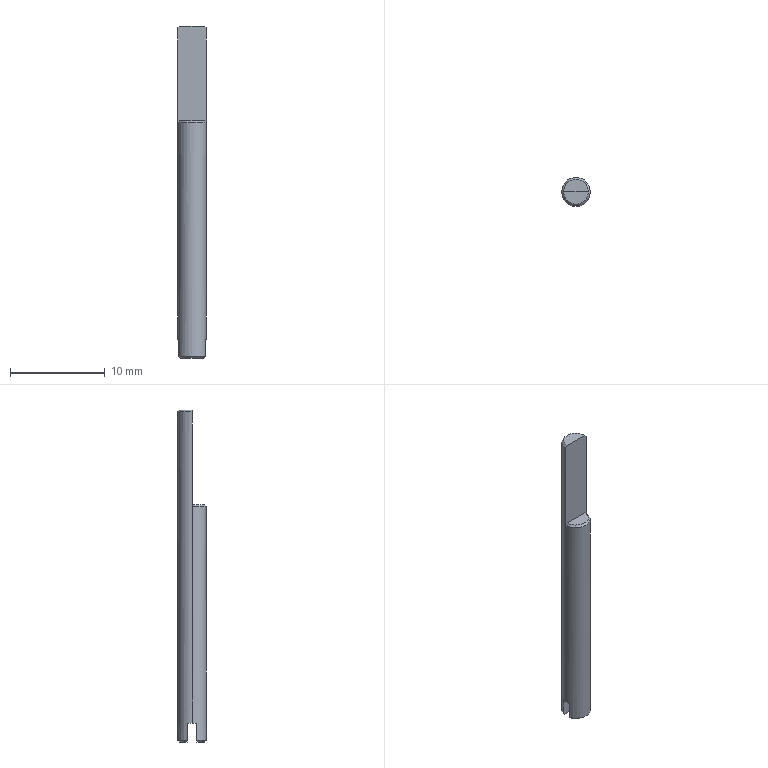Part | SolidWorks | features ICE 2, Chamfer 1, Extrusion 1 | 1 solid | 14 faces | box 3 x 3 x 35 mm | volume 205.851 mm3 | plane 8 | cone 4 | cylinder 2 | commonest cylinder face diameters 3 x2
STEP:
#1=CARTESIAN_POINT('',(1.5,0.,7.3));
#2=VERTEX_POINT('',#1);
#3=CARTESIAN_POINT('',(1.5,0.,17.3));
#4=VERTEX_POINT('',#3);
#5=CARTESIAN_POINT('',(1.5,0.,7.5));
#6=DIRECTION('',(0.,0.,1.));
#7=VECTOR('',#6,1000.);
#8=LINE('',#5,#7);
#9=EDGE_CURVE('',#2,#4,#8,.T.);
#10=ORIENTED_EDGE('',*,*,#9,.F.);
#11=CARTESIAN_POINT('',(1.5,0.,-15.5));
#12=VERTEX_POINT('',#11);
#13=CARTESIAN_POINT('',(1.5,0.,17.5));
#14=DIRECTION('',(0.,0.,-1.));
#15=VECTOR('',#14,1000.);
#16=LINE('',#13,#15);
#17=EDGE_CURVE('',#2,#12,#16,.T.);
#18=ORIENTED_EDGE('',*,*,#17,.T.);
#19=CARTESIAN_POINT('',(1.414,0.5,-15.5));
#20=VERTEX_POINT('',#19);
#21=CARTESIAN_POINT('',(0.,0.,-15.5));
#22=DIRECTION('',(0.,0.,-1.));
#23=DIRECTION('',(-1.,0.,0.));
#24=AXIS2_PLACEMENT_3D('',#21,#22,#23);
#25=CIRCLE('',#24,1.5);
#26=EDGE_CURVE('',#20,#12,#25,.T.);
#27=ORIENTED_EDGE('',*,*,#26,.F.);
#28=CARTESIAN_POINT('',(1.414,0.5,-17.3));
#29=VERTEX_POINT('',#28);
#30=CARTESIAN_POINT('',(1.414,0.5,17.5));
#31=DIRECTION('',(0.,0.,-1.));
#32=VECTOR('',#31,1000.);
#33=LINE('',#30,#32);
#34=EDGE_CURVE('',#20,#29,#33,.T.);
#35=ORIENTED_EDGE('',*,*,#34,.T.);
#36=CARTESIAN_POINT('',(-1.414,0.5,-17.3));
#37=VERTEX_POINT('',#36);
#38=CARTESIAN_POINT('',(0.,0.,-17.3));
#39=DIRECTION('',(0.,0.,1.));
#40=DIRECTION('',(1.,0.,0.));
#41=AXIS2_PLACEMENT_3D('',#38,#39,#40);
#42=CIRCLE('',#41,1.5);
#43=EDGE_CURVE('',#29,#37,#42,.T.);
#44=ORIENTED_EDGE('',*,*,#43,.T.);
#45=CARTESIAN_POINT('',(-1.414,0.5,-15.5));
#46=VERTEX_POINT('',#45);
#47=CARTESIAN_POINT('',(-1.414,0.5,17.5));
#48=DIRECTION('',(0.,0.,1.));
#49=VECTOR('',#48,1000.);
#50=LINE('',#47,#49);
#51=EDGE_CURVE('',#37,#46,#50,.T.);
#52=ORIENTED_EDGE('',*,*,#51,.T.);
#53=CARTESIAN_POINT('',(-1.5,0.,-15.5));
#54=VERTEX_POINT('',#53);
#55=CARTESIAN_POINT('',(0.,0.,-15.5));
#56=DIRECTION('',(0.,0.,-1.));
#57=DIRECTION('',(-1.,0.,0.));
#58=AXIS2_PLACEMENT_3D('',#55,#56,#57);
#59=CIRCLE('',#58,1.5);
#60=EDGE_CURVE('',#54,#46,#59,.T.);
#61=ORIENTED_EDGE('',*,*,#60,.F.);
#62=CARTESIAN_POINT('',(-1.5,0.,7.3));
#63=VERTEX_POINT('',#62);
#64=CARTESIAN_POINT('',(-1.5,0.,17.5));
#65=DIRECTION('',(0.,0.,-1.));
#66=VECTOR('',#65,1000.);
#67=LINE('',#64,#66);
#68=EDGE_CURVE('',#63,#54,#67,.T.);
#69=ORIENTED_EDGE('',*,*,#68,.F.);
#70=CARTESIAN_POINT('',(-1.5,0.,17.3));
#71=VERTEX_POINT('',#70);
#72=CARTESIAN_POINT('',(-1.5,0.,7.5));
#73=DIRECTION('',(0.,0.,1.));
#74=VECTOR('',#73,1000.);
#75=LINE('',#72,#74);
#76=EDGE_CURVE('',#63,#71,#75,.T.);
#77=ORIENTED_EDGE('',*,*,#76,.T.);
#78=CARTESIAN_POINT('',(0.,0.,17.3));
#79=DIRECTION('',(0.,0.,-1.));
#80=DIRECTION('',(1.,0.,0.));
#81=AXIS2_PLACEMENT_3D('',#78,#79,#80);
#82=CIRCLE('',#81,1.5);
#83=EDGE_CURVE('',#71,#4,#82,.T.);
#84=ORIENTED_EDGE('',*,*,#83,.T.);
#85=EDGE_LOOP('',(#10,#18,#27,#35,#44,#52,#61,#69,#77,#84));
#86=FACE_OUTER_BOUND('',#85,.T.);
#87=CARTESIAN_POINT('',(0.,0.,17.5));
#88=DIRECTION('',(0.,0.,-1.));
#89=DIRECTION('',(-1.,0.,0.));
#90=AXIS2_PLACEMENT_3D('',#87,#88,#89);
#91=CYLINDRICAL_SURFACE('',#90,1.5);
#92=ADVANCED_FACE('',(#86),#91,.T.);
#93=CARTESIAN_POINT('',(1.2,0.5,-17.5));
#94=VERTEX_POINT('',#93);
#95=CARTESIAN_POINT('',(-1.2,0.5,-17.5));
#96=VERTEX_POINT('',#95);
#97=CARTESIAN_POINT('',(0.,0.5,-17.5));
#98=DIRECTION('',(-1.,0.,0.));
#99=VECTOR('',#98,1000.);
#100=LINE('',#97,#99);
#101=EDGE_CURVE('',#94,#96,#100,.T.);
#102=ORIENTED_EDGE('',*,*,#101,.T.);
#103=CARTESIAN_POINT('',(0.,0.,-17.5));
#104=DIRECTION('',(0.,0.,-1.));
#105=DIRECTION('',(1.,0.,0.));
#106=AXIS2_PLACEMENT_3D('',#103,#104,#105);
#107=CIRCLE('',#106,1.3);
#108=EDGE_CURVE('',#96,#94,#107,.T.);
#109=ORIENTED_EDGE('',*,*,#108,.T.);
#110=EDGE_LOOP('',(#102,#109));
#111=FACE_OUTER_BOUND('',#110,.T.);
#112=CARTESIAN_POINT('',(0.,0.,-17.5));
#113=DIRECTION('',(0.,0.,1.));
#114=DIRECTION('',(1.,0.,0.));
#115=AXIS2_PLACEMENT_3D('',#112,#113,#114);
#116=PLANE('',#115);
#117=ADVANCED_FACE('',(#111),#116,.F.);
#118=ORIENTED_EDGE('',*,*,#17,.F.);
#119=CARTESIAN_POINT('',(0.,0.,7.3));
#120=DIRECTION('',(0.,0.,-1.));
#121=DIRECTION('',(-1.,0.,0.));
#122=AXIS2_PLACEMENT_3D('',#119,#120,#121);
#123=CIRCLE('',#122,1.5);
#124=EDGE_CURVE('',#2,#63,#123,.T.);
#125=ORIENTED_EDGE('',*,*,#124,.T.);
#126=ORIENTED_EDGE('',*,*,#68,.T.);
#127=CARTESIAN_POINT('',(-1.414,-0.5,-15.5));
#128=VERTEX_POINT('',#127);
#129=CARTESIAN_POINT('',(0.,0.,-15.5));
#130=DIRECTION('',(0.,0.,-1.));
#131=DIRECTION('',(-1.,0.,0.));
#132=AXIS2_PLACEMENT_3D('',#129,#130,#131);
#133=CIRCLE('',#132,1.5);
#134=EDGE_CURVE('',#128,#54,#133,.T.);
#135=ORIENTED_EDGE('',*,*,#134,.F.);
#136=CARTESIAN_POINT('',(-1.414,-0.5,-17.3));
#137=VERTEX_POINT('',#136);
#138=CARTESIAN_POINT('',(-1.414,-0.5,17.5));
#139=DIRECTION('',(0.,0.,-1.));
#140=VECTOR('',#139,1000.);
#141=LINE('',#138,#140);
#142=EDGE_CURVE('',#128,#137,#141,.T.);
#143=ORIENTED_EDGE('',*,*,#142,.T.);
#144=CARTESIAN_POINT('',(1.414,-0.5,-17.3));
#145=VERTEX_POINT('',#144);
#146=CARTESIAN_POINT('',(0.,0.,-17.3));
#147=DIRECTION('',(0.,0.,1.));
#148=DIRECTION('',(1.,0.,0.));
#149=AXIS2_PLACEMENT_3D('',#146,#147,#148);
#150=CIRCLE('',#149,1.5);
#151=EDGE_CURVE('',#137,#145,#150,.T.);
#152=ORIENTED_EDGE('',*,*,#151,.T.);
#153=CARTESIAN_POINT('',(1.414,-0.5,-15.5));
#154=VERTEX_POINT('',#153);
#155=CARTESIAN_POINT('',(1.414,-0.5,17.5));
#156=DIRECTION('',(0.,0.,1.));
#157=VECTOR('',#156,1000.);
#158=LINE('',#155,#157);
#159=EDGE_CURVE('',#145,#154,#158,.T.);
#160=ORIENTED_EDGE('',*,*,#159,.T.);
#161=CARTESIAN_POINT('',(0.,0.,-15.5));
#162=DIRECTION('',(0.,0.,-1.));
#163=DIRECTION('',(-1.,0.,0.));
#164=AXIS2_PLACEMENT_3D('',#161,#162,#163);
#165=CIRCLE('',#164,1.5);
#166=EDGE_CURVE('',#12,#154,#165,.T.);
#167=ORIENTED_EDGE('',*,*,#166,.F.);
#168=EDGE_LOOP('',(#118,#125,#126,#135,#143,#152,#160,#167));
#169=FACE_OUTER_BOUND('',#168,.T.);
#170=CARTESIAN_POINT('',(0.,0.,17.5));
#171=DIRECTION('',(0.,0.,-1.));
#172=DIRECTION('',(-1.,0.,0.));
#173=AXIS2_PLACEMENT_3D('',#170,#171,#172);
#174=CYLINDRICAL_SURFACE('',#173,1.5);
#175=ADVANCED_FACE('',(#169),#174,.T.);
#176=CARTESIAN_POINT('',(1.3,0.,17.5));
#177=VERTEX_POINT('',#176);
#178=CARTESIAN_POINT('',(-1.3,0.,17.5));
#179=VERTEX_POINT('',#178);
#180=CARTESIAN_POINT('',(1.5,0.,17.5));
#181=DIRECTION('',(-1.,0.,0.));
#182=VECTOR('',#181,1000.);
#183=LINE('',#180,#182);
#184=EDGE_CURVE('',#177,#179,#183,.T.);
#185=ORIENTED_EDGE('',*,*,#184,.F.);
#186=CARTESIAN_POINT('',(0.,0.,17.5));
#187=DIRECTION('',(0.,0.,1.));
#188=DIRECTION('',(1.,0.,0.));
#189=AXIS2_PLACEMENT_3D('',#186,#187,#188);
#190=CIRCLE('',#189,1.3);
#191=EDGE_CURVE('',#177,#179,#190,.T.);
#192=ORIENTED_EDGE('',*,*,#191,.T.);
#193=EDGE_LOOP('',(#185,#192));
#194=FACE_OUTER_BOUND('',#193,.T.);
#195=CARTESIAN_POINT('',(0.,0.,17.5));
#196=DIRECTION('',(0.,0.,1.));
#197=DIRECTION('',(1.,0.,0.));
#198=AXIS2_PLACEMENT_3D('',#195,#196,#197);
#199=PLANE('',#198);
#200=ADVANCED_FACE('',(#194),#199,.T.);
#201=CARTESIAN_POINT('',(-1.2,-0.5,-17.5));
#202=VERTEX_POINT('',#201);
#203=CARTESIAN_POINT('',(1.2,-0.5,-17.5));
#204=VERTEX_POINT('',#203);
#205=CARTESIAN_POINT('',(0.,-0.5,-17.5));
#206=DIRECTION('',(1.,0.,0.));
#207=VECTOR('',#206,1000.);
#208=LINE('',#205,#207);
#209=EDGE_CURVE('',#202,#204,#208,.T.);
#210=ORIENTED_EDGE('',*,*,#209,.T.);
#211=CARTESIAN_POINT('',(0.,0.,-17.5));
#212=DIRECTION('',(0.,0.,-1.));
#213=DIRECTION('',(1.,0.,0.));
#214=AXIS2_PLACEMENT_3D('',#211,#212,#213);
#215=CIRCLE('',#214,1.3);
#216=EDGE_CURVE('',#204,#202,#215,.T.);
#217=ORIENTED_EDGE('',*,*,#216,.T.);
#218=EDGE_LOOP('',(#210,#217));
#219=FACE_OUTER_BOUND('',#218,.T.);
#220=CARTESIAN_POINT('',(0.,0.,-17.5));
#221=DIRECTION('',(0.,0.,1.));
#222=DIRECTION('',(1.,0.,0.));
#223=AXIS2_PLACEMENT_3D('',#220,#221,#222);
#224=PLANE('',#223);
#225=ADVANCED_FACE('',(#219),#224,.F.);
#226=CARTESIAN_POINT('',(1.3,0.,7.5));
#227=VERTEX_POINT('',#226);
#228=CARTESIAN_POINT('',(-1.3,0.,7.5));
#229=VERTEX_POINT('',#228);
#230=CARTESIAN_POINT('',(1.5,0.,7.5));
#231=DIRECTION('',(-1.,0.,0.));
#232=VECTOR('',#231,1000.);
#233=LINE('',#230,#232);
#234=EDGE_CURVE('',#227,#229,#233,.T.);
#235=ORIENTED_EDGE('',*,*,#234,.T.);
#236=CARTESIAN_POINT('',(0.,0.,7.5));
#237=DIRECTION('',(0.,0.,1.));
#238=DIRECTION('',(-1.,0.,0.));
#239=AXIS2_PLACEMENT_3D('',#236,#237,#238);
#240=CIRCLE('',#239,1.3);
#241=EDGE_CURVE('',#229,#227,#240,.T.);
#242=ORIENTED_EDGE('',*,*,#241,.T.);
#243=EDGE_LOOP('',(#235,#242));
#244=FACE_OUTER_BOUND('',#243,.T.);
#245=CARTESIAN_POINT('',(0.,0.,7.5));
#246=DIRECTION('',(0.,0.,-1.));
#247=DIRECTION('',(-1.,0.,0.));
#248=AXIS2_PLACEMENT_3D('',#245,#246,#247);
#249=PLANE('',#248);
#250=ADVANCED_FACE('',(#244),#249,.F.);
#251=ORIENTED_EDGE('',*,*,#184,.T.);
#252=CARTESIAN_POINT('',(0.,0.,18.8));
#253=DIRECTION('',(-0.7071,0.,-0.7071));
#254=VECTOR('',#253,1000.);
#255=LINE('',#252,#254);
#256=EDGE_CURVE('',#179,#71,#255,.T.);
#257=ORIENTED_EDGE('',*,*,#256,.T.);
#258=ORIENTED_EDGE('',*,*,#76,.F.);
#259=CARTESIAN_POINT('',(0.,0.,8.8));
#260=DIRECTION('',(0.7071,0.,0.7071));
#261=VECTOR('',#260,1000.);
#262=LINE('',#259,#261);
#263=EDGE_CURVE('',#63,#229,#262,.T.);
#264=ORIENTED_EDGE('',*,*,#263,.T.);
#265=ORIENTED_EDGE('',*,*,#234,.F.);
#266=CARTESIAN_POINT('',(0.,0.,8.8));
#267=DIRECTION('',(0.7071,0.,-0.7071));
#268=VECTOR('',#267,1000.);
#269=LINE('',#266,#268);
#270=EDGE_CURVE('',#227,#2,#269,.T.);
#271=ORIENTED_EDGE('',*,*,#270,.T.);
#272=ORIENTED_EDGE('',*,*,#9,.T.);
#273=CARTESIAN_POINT('',(0.,0.,18.8));
#274=DIRECTION('',(-0.7071,0.,0.7071));
#275=VECTOR('',#274,1000.);
#276=LINE('',#273,#275);
#277=EDGE_CURVE('',#4,#177,#276,.T.);
#278=ORIENTED_EDGE('',*,*,#277,.T.);
#279=EDGE_LOOP('',(#251,#257,#258,#264,#265,#271,#272,#278));
#280=FACE_OUTER_BOUND('',#279,.T.);
#281=CARTESIAN_POINT('',(1.5,0.,7.5));
#282=DIRECTION('',(0.,1.,0.));
#283=DIRECTION('',(0.,0.,1.));
#284=AXIS2_PLACEMENT_3D('',#281,#282,#283);
#285=PLANE('',#284);
#286=ADVANCED_FACE('',(#280),#285,.F.);
#287=ORIENTED_EDGE('',*,*,#26,.T.);
#288=ORIENTED_EDGE('',*,*,#166,.T.);
#289=CARTESIAN_POINT('',(-2.348,-0.5,-15.5));
#290=DIRECTION('',(-1.,0.,0.));
#291=VECTOR('',#290,1000.);
#292=LINE('',#289,#291);
#293=EDGE_CURVE('',#154,#128,#292,.T.);
#294=ORIENTED_EDGE('',*,*,#293,.T.);
#295=ORIENTED_EDGE('',*,*,#134,.T.);
#296=ORIENTED_EDGE('',*,*,#60,.T.);
#297=CARTESIAN_POINT('',(-2.348,0.5,-15.5));
#298=DIRECTION('',(1.,0.,0.));
#299=VECTOR('',#298,1000.);
#300=LINE('',#297,#299);
#301=EDGE_CURVE('',#46,#20,#300,.T.);
#302=ORIENTED_EDGE('',*,*,#301,.T.);
#303=EDGE_LOOP('',(#287,#288,#294,#295,#296,#302));
#304=FACE_OUTER_BOUND('',#303,.T.);
#305=CARTESIAN_POINT('',(0.,0.,-15.5));
#306=DIRECTION('',(0.,0.,-1.));
#307=DIRECTION('',(-1.,0.,0.));
#308=AXIS2_PLACEMENT_3D('',#305,#306,#307);
#309=PLANE('',#308);
#310=ADVANCED_FACE('',(#304),#309,.T.);
#311=ORIENTED_EDGE('',*,*,#51,.F.);
#312=CARTESIAN_POINT('',(-1.414,0.5,-17.3));
#313=CARTESIAN_POINT('',(-1.343,0.5,-17.367));
#314=CARTESIAN_POINT('',(-1.272,0.5,-17.434));
#315=CARTESIAN_POINT('',(-1.2,0.5,-17.5));
#316=B_SPLINE_CURVE_WITH_KNOTS('',3,(#312,#313,#314,#315),.UNSPECIFIED.,.F.,.F.,(4,4),(0.,0.0002931),.UNSPECIFIED.);
#317=EDGE_CURVE('',#37,#96,#316,.T.);
#318=ORIENTED_EDGE('',*,*,#317,.T.);
#319=ORIENTED_EDGE('',*,*,#101,.F.);
#320=CARTESIAN_POINT('',(1.2,0.5,-17.5));
#321=CARTESIAN_POINT('',(1.272,0.5,-17.434));
#322=CARTESIAN_POINT('',(1.343,0.5,-17.367));
#323=CARTESIAN_POINT('',(1.414,0.5,-17.3));
#324=B_SPLINE_CURVE_WITH_KNOTS('',3,(#320,#321,#322,#323),.UNSPECIFIED.,.F.,.F.,(4,4),(0.,0.0002931),.UNSPECIFIED.);
#325=EDGE_CURVE('',#94,#29,#324,.T.);
#326=ORIENTED_EDGE('',*,*,#325,.T.);
#327=ORIENTED_EDGE('',*,*,#34,.F.);
#328=ORIENTED_EDGE('',*,*,#301,.F.);
#329=EDGE_LOOP('',(#311,#318,#319,#326,#327,#328));
#330=FACE_OUTER_BOUND('',#329,.T.);
#331=CARTESIAN_POINT('',(-2.348,0.5,-15.5));
#332=DIRECTION('',(0.,1.,0.));
#333=DIRECTION('',(-1.,0.,0.));
#334=AXIS2_PLACEMENT_3D('',#331,#332,#333);
#335=PLANE('',#334);
#336=ADVANCED_FACE('',(#330),#335,.F.);
#337=ORIENTED_EDGE('',*,*,#159,.F.);
#338=CARTESIAN_POINT('',(1.414,-0.5,-17.3));
#339=CARTESIAN_POINT('',(1.343,-0.5,-17.367));
#340=CARTESIAN_POINT('',(1.272,-0.5,-17.434));
#341=CARTESIAN_POINT('',(1.2,-0.5,-17.5));
#342=B_SPLINE_CURVE_WITH_KNOTS('',3,(#338,#339,#340,#341),.UNSPECIFIED.,.F.,.F.,(4,4),(0.,0.0002931),.UNSPECIFIED.);
#343=EDGE_CURVE('',#145,#204,#342,.T.);
#344=ORIENTED_EDGE('',*,*,#343,.T.);
#345=ORIENTED_EDGE('',*,*,#209,.F.);
#346=CARTESIAN_POINT('',(-1.2,-0.5,-17.5));
#347=CARTESIAN_POINT('',(-1.272,-0.5,-17.434));
#348=CARTESIAN_POINT('',(-1.343,-0.5,-17.367));
#349=CARTESIAN_POINT('',(-1.414,-0.5,-17.3));
#350=B_SPLINE_CURVE_WITH_KNOTS('',3,(#346,#347,#348,#349),.UNSPECIFIED.,.F.,.F.,(4,4),(0.,0.0002931),.UNSPECIFIED.);
#351=EDGE_CURVE('',#202,#137,#350,.T.);
#352=ORIENTED_EDGE('',*,*,#351,.T.);
#353=ORIENTED_EDGE('',*,*,#142,.F.);
#354=ORIENTED_EDGE('',*,*,#293,.F.);
#355=EDGE_LOOP('',(#337,#344,#345,#352,#353,#354));
#356=FACE_OUTER_BOUND('',#355,.T.);
#357=CARTESIAN_POINT('',(-2.348,-0.5,-15.5));
#358=DIRECTION('',(0.,-1.,0.));
#359=DIRECTION('',(1.,0.,0.));
#360=AXIS2_PLACEMENT_3D('',#357,#358,#359);
#361=PLANE('',#360);
#362=ADVANCED_FACE('',(#356),#361,.F.);
#363=ORIENTED_EDGE('',*,*,#325,.F.);
#364=ORIENTED_EDGE('',*,*,#108,.F.);
#365=ORIENTED_EDGE('',*,*,#317,.F.);
#366=ORIENTED_EDGE('',*,*,#43,.F.);
#367=EDGE_LOOP('',(#363,#364,#365,#366));
#368=FACE_OUTER_BOUND('',#367,.T.);
#369=CARTESIAN_POINT('',(0.,0.,-17.3));
#370=DIRECTION('',(0.,0.,1.));
#371=DIRECTION('',(1.,0.,0.));
#372=AXIS2_PLACEMENT_3D('',#369,#370,#371);
#373=CONICAL_SURFACE('',#372,1.5,0.7854);
#374=ADVANCED_FACE('',(#368),#373,.T.);
#375=ORIENTED_EDGE('',*,*,#351,.F.);
#376=ORIENTED_EDGE('',*,*,#216,.F.);
#377=ORIENTED_EDGE('',*,*,#343,.F.);
#378=ORIENTED_EDGE('',*,*,#151,.F.);
#379=EDGE_LOOP('',(#375,#376,#377,#378));
#380=FACE_OUTER_BOUND('',#379,.T.);
#381=CARTESIAN_POINT('',(0.,0.,-17.3));
#382=DIRECTION('',(0.,0.,1.));
#383=DIRECTION('',(1.,0.,0.));
#384=AXIS2_PLACEMENT_3D('',#381,#382,#383);
#385=CONICAL_SURFACE('',#384,1.5,0.7854);
#386=ADVANCED_FACE('',(#380),#385,.T.);
#387=ORIENTED_EDGE('',*,*,#277,.F.);
#388=ORIENTED_EDGE('',*,*,#83,.F.);
#389=ORIENTED_EDGE('',*,*,#256,.F.);
#390=ORIENTED_EDGE('',*,*,#191,.F.);
#391=EDGE_LOOP('',(#387,#388,#389,#390));
#392=FACE_OUTER_BOUND('',#391,.T.);
#393=CARTESIAN_POINT('',(0.,0.,17.5));
#394=DIRECTION('',(0.,0.,-1.));
#395=DIRECTION('',(-1.,0.,0.));
#396=AXIS2_PLACEMENT_3D('',#393,#394,#395);
#397=CONICAL_SURFACE('',#396,1.3,0.7854);
#398=ADVANCED_FACE('',(#392),#397,.T.);
#399=ORIENTED_EDGE('',*,*,#270,.F.);
#400=ORIENTED_EDGE('',*,*,#241,.F.);
#401=ORIENTED_EDGE('',*,*,#263,.F.);
#402=ORIENTED_EDGE('',*,*,#124,.F.);
#403=EDGE_LOOP('',(#399,#400,#401,#402));
#404=FACE_OUTER_BOUND('',#403,.T.);
#405=CARTESIAN_POINT('',(0.,0.,7.3));
#406=DIRECTION('',(0.,0.,-1.));
#407=DIRECTION('',(-1.,0.,0.));
#408=AXIS2_PLACEMENT_3D('',#405,#406,#407);
#409=CONICAL_SURFACE('',#408,1.5,0.7854);
#410=ADVANCED_FACE('',(#404),#409,.T.);
#411=CLOSED_SHELL('',(#92,#117,#175,#200,#225,#250,#286,#310,#336,#362,#374,#386,#398,#410));
#412=MANIFOLD_SOLID_BREP('',#411);
#413=CARTESIAN_POINT('',(0.,0.,0.));
#414=DIRECTION('',(0.,0.,1.));
#415=DIRECTION('',(1.,0.,0.));
#416=AXIS2_PLACEMENT_3D('',#413,#414,#415);
#417=(LENGTH_UNIT()NAMED_UNIT(*)SI_UNIT(.MILLI.,.METRE.));
#418=UNCERTAINTY_MEASURE_WITH_UNIT(LENGTH_MEASURE(0.00001),#417,'','');
#419=(NAMED_UNIT(*)PLANE_ANGLE_UNIT()SI_UNIT($,.RADIAN.));
#420=(NAMED_UNIT(*)SI_UNIT($,.STERADIAN.)SOLID_ANGLE_UNIT());
#421=(GEOMETRIC_REPRESENTATION_CONTEXT(3)GLOBAL_UNCERTAINTY_ASSIGNED_CONTEXT((#418))GLOBAL_UNIT_ASSIGNED_CONTEXT((#417,#419,#420))REPRESENTATION_CONTEXT('',''));
#422=ADVANCED_BREP_SHAPE_REPRESENTATION('',(#412,#416),#421);